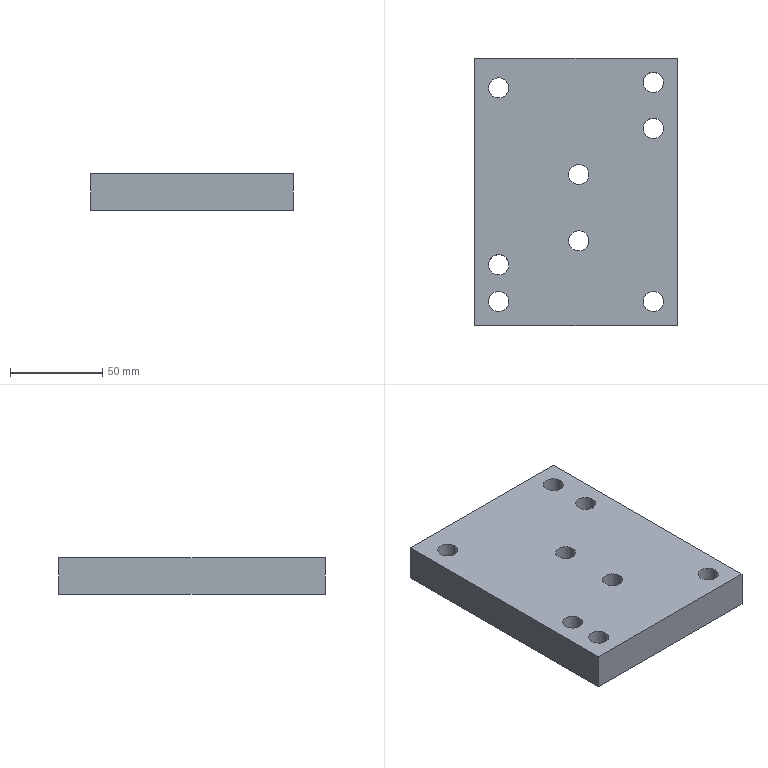Part | STEP file | 109_id3170_x_t | 1 solid | 14 faces | box 110 x 145 x 20 mm | volume 303795 mm3 | cylinder 8 | plane 6 | commonest cylinder face diameters 11 x8
STEP:
#1=CARTESIAN_POINT('',(0.,0.,0.));
#2=DIRECTION('',(0.,0.,1.));
#3=DIRECTION('',(1.,0.,0.));
#4=AXIS2_PLACEMENT_3D('',#1,#2,#3);
#5=CARTESIAN_POINT('',(-312.,-123.,105.));
#6=VERTEX_POINT('',#5);
#7=CARTESIAN_POINT('',(-317.5,-123.,105.));
#8=DIRECTION('',(0.,0.,1.));
#9=DIRECTION('',(1.,0.,0.));
#10=AXIS2_PLACEMENT_3D('',#7,#8,#9);
#11=CIRCLE('',#10,5.5);
#12=CARTESIAN_POINT('',(-319.,-95.5,105.));
#13=DIRECTION('',(0.,0.,1.));
#14=DIRECTION('',(-1.,0.,0.));
#15=AXIS2_PLACEMENT_3D('',#12,#13,#14);
#16=PLANE('',#15);
#17=CARTESIAN_POINT('',(-1.5,27.5));
#18=DIRECTION('',(-1.,0.));
#19=AXIS2_PLACEMENT_2D('',#17,#18);
#20=CIRCLE('',#19,5.5);
#21=(GEOMETRIC_REPRESENTATION_CONTEXT(2)PARAMETRIC_REPRESENTATION_CONTEXT()REPRESENTATION_CONTEXT('',''));
#22=DEFINITIONAL_REPRESENTATION('',(#20),#21);
#23=PCURVE('',#16,#22);
#24=CARTESIAN_POINT('',(-317.5,-123.,289.));
#25=DIRECTION('',(0.,0.,-1.));
#26=DIRECTION('',(1.,0.,0.));
#27=AXIS2_PLACEMENT_3D('',#24,#25,#26);
#28=CYLINDRICAL_SURFACE('',#27,5.5);
#29=CARTESIAN_POINT('',(6.283,184.));
#30=DIRECTION('',(-1.,0.));
#31=VECTOR('',#30,1.);
#32=LINE('',#29,#31);
#33=(GEOMETRIC_REPRESENTATION_CONTEXT(2)PARAMETRIC_REPRESENTATION_CONTEXT()REPRESENTATION_CONTEXT('',''));
#34=DEFINITIONAL_REPRESENTATION('',(#32),#33);
#35=PCURVE('',#28,#34);
#36=SURFACE_CURVE('',#11,(#23,#35),.PCURVE_S1.);
#37=EDGE_CURVE('',#6,#6,#36,.T.);
#38=ORIENTED_EDGE('',*,*,#37,.F.);
#39=EDGE_LOOP('',(#38));
#40=FACE_BOUND('',#39,.T.);
#41=CARTESIAN_POINT('',(-312.,-87.,105.));
#42=VERTEX_POINT('',#41);
#43=CARTESIAN_POINT('',(-317.5,-87.,105.));
#44=DIRECTION('',(0.,0.,1.));
#45=DIRECTION('',(1.,0.,0.));
#46=AXIS2_PLACEMENT_3D('',#43,#44,#45);
#47=CIRCLE('',#46,5.5);
#48=CARTESIAN_POINT('',(-1.5,-8.5));
#49=DIRECTION('',(-1.,0.));
#50=AXIS2_PLACEMENT_2D('',#48,#49);
#51=CIRCLE('',#50,5.5);
#52=(GEOMETRIC_REPRESENTATION_CONTEXT(2)PARAMETRIC_REPRESENTATION_CONTEXT()REPRESENTATION_CONTEXT('',''));
#53=DEFINITIONAL_REPRESENTATION('',(#51),#52);
#54=PCURVE('',#16,#53);
#55=CARTESIAN_POINT('',(-317.5,-87.,289.));
#56=DIRECTION('',(0.,0.,-1.));
#57=DIRECTION('',(1.,0.,0.));
#58=AXIS2_PLACEMENT_3D('',#55,#56,#57);
#59=CYLINDRICAL_SURFACE('',#58,5.5);
#60=CARTESIAN_POINT('',(6.283,184.));
#61=DIRECTION('',(-1.,0.));
#62=VECTOR('',#61,1.);
#63=LINE('',#60,#62);
#64=(GEOMETRIC_REPRESENTATION_CONTEXT(2)PARAMETRIC_REPRESENTATION_CONTEXT()REPRESENTATION_CONTEXT('',''));
#65=DEFINITIONAL_REPRESENTATION('',(#63),#64);
#66=PCURVE('',#59,#65);
#67=SURFACE_CURVE('',#47,(#54,#66),.PCURVE_S1.);
#68=EDGE_CURVE('',#42,#42,#67,.T.);
#69=ORIENTED_EDGE('',*,*,#68,.F.);
#70=EDGE_LOOP('',(#69));
#71=FACE_BOUND('',#70,.T.);
#72=CARTESIAN_POINT('',(-355.5,-136.,105.));
#73=VERTEX_POINT('',#72);
#74=CARTESIAN_POINT('',(-361.,-136.,105.));
#75=DIRECTION('',(0.,0.,-1.));
#76=DIRECTION('',(1.,0.,0.));
#77=AXIS2_PLACEMENT_3D('',#74,#75,#76);
#78=CIRCLE('',#77,5.5);
#79=CARTESIAN_POINT('',(36.5,40.5));
#80=CARTESIAN_POINT('',(36.5,50.026));
#81=CARTESIAN_POINT('',(44.75,45.263));
#82=CARTESIAN_POINT('',(53.,40.5));
#83=CARTESIAN_POINT('',(44.75,35.737));
#84=CARTESIAN_POINT('',(36.5,30.974));
#85=CARTESIAN_POINT('',(36.5,40.5));
#86=(BOUNDED_CURVE()B_SPLINE_CURVE(2,(#79,#80,#81,#82,#83,#84,#85),.UNSPECIFIED.,.T.,.F.)B_SPLINE_CURVE_WITH_KNOTS((1,2,2,2,2,1),(-2.094,0.,2.094,4.189,6.283,8.378),.UNSPECIFIED.)CURVE()GEOMETRIC_REPRESENTATION_ITEM()RATIONAL_B_SPLINE_CURVE((1.,0.5,1.,0.5,1.,0.5,1.))REPRESENTATION_ITEM(''));
#87=(GEOMETRIC_REPRESENTATION_CONTEXT(2)PARAMETRIC_REPRESENTATION_CONTEXT()REPRESENTATION_CONTEXT('',''));
#88=DEFINITIONAL_REPRESENTATION('',(#86),#87);
#89=PCURVE('',#16,#88);
#90=CARTESIAN_POINT('',(-361.,-136.,90.));
#91=DIRECTION('',(0.,0.,1.));
#92=DIRECTION('',(-1.,0.,0.));
#93=AXIS2_PLACEMENT_3D('',#90,#91,#92);
#94=CYLINDRICAL_SURFACE('',#93,5.5);
#95=CARTESIAN_POINT('',(9.425,15.));
#96=DIRECTION('',(-1.,0.));
#97=VECTOR('',#96,1.);
#98=LINE('',#95,#97);
#99=(GEOMETRIC_REPRESENTATION_CONTEXT(2)PARAMETRIC_REPRESENTATION_CONTEXT()REPRESENTATION_CONTEXT('',''));
#100=DEFINITIONAL_REPRESENTATION('',(#98),#99);
#101=PCURVE('',#94,#100);
#102=SURFACE_CURVE('',#78,(#89,#101),.PCURVE_S1.);
#103=EDGE_CURVE('',#73,#73,#102,.T.);
#104=ORIENTED_EDGE('',*,*,#103,.T.);
#105=EDGE_LOOP('',(#104));
#106=FACE_BOUND('',#105,.T.);
#107=CARTESIAN_POINT('',(-271.5,-37.,105.));
#108=VERTEX_POINT('',#107);
#109=CARTESIAN_POINT('',(-277.,-37.,105.));
#110=DIRECTION('',(0.,0.,-1.));
#111=DIRECTION('',(1.,0.,0.));
#112=AXIS2_PLACEMENT_3D('',#109,#110,#111);
#113=CIRCLE('',#112,5.5);
#114=CARTESIAN_POINT('',(-47.5,-58.5));
#115=CARTESIAN_POINT('',(-47.5,-48.974));
#116=CARTESIAN_POINT('',(-39.25,-53.737));
#117=CARTESIAN_POINT('',(-31.,-58.5));
#118=CARTESIAN_POINT('',(-39.25,-63.263));
#119=CARTESIAN_POINT('',(-47.5,-68.026));
#120=CARTESIAN_POINT('',(-47.5,-58.5));
#121=(BOUNDED_CURVE()B_SPLINE_CURVE(2,(#114,#115,#116,#117,#118,#119,#120),.UNSPECIFIED.,.T.,.F.)B_SPLINE_CURVE_WITH_KNOTS((1,2,2,2,2,1),(-2.094,0.,2.094,4.189,6.283,8.378),.UNSPECIFIED.)CURVE()GEOMETRIC_REPRESENTATION_ITEM()RATIONAL_B_SPLINE_CURVE((1.,0.5,1.,0.5,1.,0.5,1.))REPRESENTATION_ITEM(''));
#122=(GEOMETRIC_REPRESENTATION_CONTEXT(2)PARAMETRIC_REPRESENTATION_CONTEXT()REPRESENTATION_CONTEXT('',''));
#123=DEFINITIONAL_REPRESENTATION('',(#121),#122);
#124=PCURVE('',#16,#123);
#125=CARTESIAN_POINT('',(-277.,-37.,90.));
#126=DIRECTION('',(0.,0.,1.));
#127=DIRECTION('',(-1.,0.,0.));
#128=AXIS2_PLACEMENT_3D('',#125,#126,#127);
#129=CYLINDRICAL_SURFACE('',#128,5.5);
#130=CARTESIAN_POINT('',(9.425,15.));
#131=DIRECTION('',(-1.,0.));
#132=VECTOR('',#131,1.);
#133=LINE('',#130,#132);
#134=(GEOMETRIC_REPRESENTATION_CONTEXT(2)PARAMETRIC_REPRESENTATION_CONTEXT()REPRESENTATION_CONTEXT('',''));
#135=DEFINITIONAL_REPRESENTATION('',(#133),#134);
#136=PCURVE('',#129,#135);
#137=SURFACE_CURVE('',#113,(#124,#136),.PCURVE_S1.);
#138=EDGE_CURVE('',#108,#108,#137,.T.);
#139=ORIENTED_EDGE('',*,*,#138,.T.);
#140=EDGE_LOOP('',(#139));
#141=FACE_BOUND('',#140,.T.);
#142=CARTESIAN_POINT('',(-355.5,-156.,105.));
#143=VERTEX_POINT('',#142);
#144=CARTESIAN_POINT('',(-361.,-156.,105.));
#145=DIRECTION('',(0.,0.,-1.));
#146=DIRECTION('',(1.,0.,0.));
#147=AXIS2_PLACEMENT_3D('',#144,#145,#146);
#148=CIRCLE('',#147,5.5);
#149=CARTESIAN_POINT('',(36.5,60.5));
#150=CARTESIAN_POINT('',(36.5,70.026));
#151=CARTESIAN_POINT('',(44.75,65.263));
#152=CARTESIAN_POINT('',(53.,60.5));
#153=CARTESIAN_POINT('',(44.75,55.737));
#154=CARTESIAN_POINT('',(36.5,50.974));
#155=CARTESIAN_POINT('',(36.5,60.5));
#156=(BOUNDED_CURVE()B_SPLINE_CURVE(2,(#149,#150,#151,#152,#153,#154,#155),.UNSPECIFIED.,.T.,.F.)B_SPLINE_CURVE_WITH_KNOTS((1,2,2,2,2,1),(-2.094,0.,2.094,4.189,6.283,8.378),.UNSPECIFIED.)CURVE()GEOMETRIC_REPRESENTATION_ITEM()RATIONAL_B_SPLINE_CURVE((1.,0.5,1.,0.5,1.,0.5,1.))REPRESENTATION_ITEM(''));
#157=(GEOMETRIC_REPRESENTATION_CONTEXT(2)PARAMETRIC_REPRESENTATION_CONTEXT()REPRESENTATION_CONTEXT('',''));
#158=DEFINITIONAL_REPRESENTATION('',(#156),#157);
#159=PCURVE('',#16,#158);
#160=CARTESIAN_POINT('',(-361.,-156.,90.));
#161=DIRECTION('',(0.,0.,1.));
#162=DIRECTION('',(-1.,0.,0.));
#163=AXIS2_PLACEMENT_3D('',#160,#161,#162);
#164=CYLINDRICAL_SURFACE('',#163,5.5);
#165=CARTESIAN_POINT('',(9.425,15.));
#166=DIRECTION('',(-1.,0.));
#167=VECTOR('',#166,1.);
#168=LINE('',#165,#167);
#169=(GEOMETRIC_REPRESENTATION_CONTEXT(2)PARAMETRIC_REPRESENTATION_CONTEXT()REPRESENTATION_CONTEXT('',''));
#170=DEFINITIONAL_REPRESENTATION('',(#168),#169);
#171=PCURVE('',#164,#170);
#172=SURFACE_CURVE('',#148,(#159,#171),.PCURVE_S1.);
#173=EDGE_CURVE('',#143,#143,#172,.T.);
#174=ORIENTED_EDGE('',*,*,#173,.T.);
#175=EDGE_LOOP('',(#174));
#176=FACE_BOUND('',#175,.T.);
#177=CARTESIAN_POINT('',(-264.,-169.,105.));
#178=VERTEX_POINT('',#177);
#179=CARTESIAN_POINT('',(-374.,-169.,105.));
#180=VERTEX_POINT('',#179);
#181=CARTESIAN_POINT('',(-319.,-169.,105.));
#182=DIRECTION('',(-1.,0.,0.));
#183=VECTOR('',#182,1.);
#184=LINE('',#181,#183);
#185=CARTESIAN_POINT('',(0.,73.5));
#186=DIRECTION('',(1.,0.));
#187=VECTOR('',#186,1.);
#188=LINE('',#185,#187);
#189=(GEOMETRIC_REPRESENTATION_CONTEXT(2)PARAMETRIC_REPRESENTATION_CONTEXT()REPRESENTATION_CONTEXT('',''));
#190=DEFINITIONAL_REPRESENTATION('',(#188),#189);
#191=PCURVE('',#16,#190);
#192=CARTESIAN_POINT('',(-319.,-169.,90.));
#193=DIRECTION('',(0.,-1.,0.));
#194=DIRECTION('',(0.,0.,1.));
#195=AXIS2_PLACEMENT_3D('',#192,#193,#194);
#196=PLANE('',#195);
#197=CARTESIAN_POINT('',(15.,0.));
#198=DIRECTION('',(0.,1.));
#199=VECTOR('',#198,1.);
#200=LINE('',#197,#199);
#201=(GEOMETRIC_REPRESENTATION_CONTEXT(2)PARAMETRIC_REPRESENTATION_CONTEXT()REPRESENTATION_CONTEXT('',''));
#202=DEFINITIONAL_REPRESENTATION('',(#200),#201);
#203=PCURVE('',#196,#202);
#204=SURFACE_CURVE('',#184,(#191,#203),.PCURVE_S1.);
#205=EDGE_CURVE('',#178,#180,#204,.T.);
#206=ORIENTED_EDGE('',*,*,#205,.F.);
#207=CARTESIAN_POINT('',(-264.,-24.,105.));
#208=VERTEX_POINT('',#207);
#209=CARTESIAN_POINT('',(-264.,-95.5,105.));
#210=DIRECTION('',(0.,-1.,0.));
#211=VECTOR('',#210,1.);
#212=LINE('',#209,#211);
#213=CARTESIAN_POINT('',(-55.,0.));
#214=DIRECTION('',(0.,1.));
#215=VECTOR('',#214,1.);
#216=LINE('',#213,#215);
#217=(GEOMETRIC_REPRESENTATION_CONTEXT(2)PARAMETRIC_REPRESENTATION_CONTEXT()REPRESENTATION_CONTEXT('',''));
#218=DEFINITIONAL_REPRESENTATION('',(#216),#217);
#219=PCURVE('',#16,#218);
#220=CARTESIAN_POINT('',(-264.,-95.5,90.));
#221=DIRECTION('',(1.,0.,0.));
#222=DIRECTION('',(0.,0.,1.));
#223=AXIS2_PLACEMENT_3D('',#220,#221,#222);
#224=PLANE('',#223);
#225=CARTESIAN_POINT('',(15.,0.));
#226=DIRECTION('',(0.,1.));
#227=VECTOR('',#226,1.);
#228=LINE('',#225,#227);
#229=(GEOMETRIC_REPRESENTATION_CONTEXT(2)PARAMETRIC_REPRESENTATION_CONTEXT()REPRESENTATION_CONTEXT('',''));
#230=DEFINITIONAL_REPRESENTATION('',(#228),#229);
#231=PCURVE('',#224,#230);
#232=SURFACE_CURVE('',#212,(#219,#231),.PCURVE_S1.);
#233=EDGE_CURVE('',#208,#178,#232,.T.);
#234=ORIENTED_EDGE('',*,*,#233,.F.);
#235=CARTESIAN_POINT('',(-374.,-24.,105.));
#236=VERTEX_POINT('',#235);
#237=CARTESIAN_POINT('',(-319.,-24.,105.));
#238=DIRECTION('',(1.,0.,0.));
#239=VECTOR('',#238,1.);
#240=LINE('',#237,#239);
#241=CARTESIAN_POINT('',(0.,-71.5));
#242=DIRECTION('',(-1.,0.));
#243=VECTOR('',#242,1.);
#244=LINE('',#241,#243);
#245=(GEOMETRIC_REPRESENTATION_CONTEXT(2)PARAMETRIC_REPRESENTATION_CONTEXT()REPRESENTATION_CONTEXT('',''));
#246=DEFINITIONAL_REPRESENTATION('',(#244),#245);
#247=PCURVE('',#16,#246);
#248=CARTESIAN_POINT('',(-319.,-24.,90.));
#249=DIRECTION('',(0.,1.,0.));
#250=DIRECTION('',(0.,0.,-1.));
#251=AXIS2_PLACEMENT_3D('',#248,#249,#250);
#252=PLANE('',#251);
#253=CARTESIAN_POINT('',(-15.,0.));
#254=DIRECTION('',(0.,-1.));
#255=VECTOR('',#254,1.);
#256=LINE('',#253,#255);
#257=(GEOMETRIC_REPRESENTATION_CONTEXT(2)PARAMETRIC_REPRESENTATION_CONTEXT()REPRESENTATION_CONTEXT('',''));
#258=DEFINITIONAL_REPRESENTATION('',(#256),#257);
#259=PCURVE('',#252,#258);
#260=SURFACE_CURVE('',#240,(#247,#259),.PCURVE_S1.);
#261=EDGE_CURVE('',#236,#208,#260,.T.);
#262=ORIENTED_EDGE('',*,*,#261,.F.);
#263=CARTESIAN_POINT('',(-374.,-95.5,105.));
#264=DIRECTION('',(0.,1.,0.));
#265=VECTOR('',#264,1.);
#266=LINE('',#263,#265);
#267=CARTESIAN_POINT('',(55.,0.));
#268=DIRECTION('',(0.,-1.));
#269=VECTOR('',#268,1.);
#270=LINE('',#267,#269);
#271=(GEOMETRIC_REPRESENTATION_CONTEXT(2)PARAMETRIC_REPRESENTATION_CONTEXT()REPRESENTATION_CONTEXT('',''));
#272=DEFINITIONAL_REPRESENTATION('',(#270),#271);
#273=PCURVE('',#16,#272);
#274=CARTESIAN_POINT('',(-374.,-95.5,90.));
#275=DIRECTION('',(-1.,0.,0.));
#276=DIRECTION('',(0.,0.,-1.));
#277=AXIS2_PLACEMENT_3D('',#274,#275,#276);
#278=PLANE('',#277);
#279=CARTESIAN_POINT('',(-15.,0.));
#280=DIRECTION('',(0.,-1.));
#281=VECTOR('',#280,1.);
#282=LINE('',#279,#281);
#283=(GEOMETRIC_REPRESENTATION_CONTEXT(2)PARAMETRIC_REPRESENTATION_CONTEXT()REPRESENTATION_CONTEXT('',''));
#284=DEFINITIONAL_REPRESENTATION('',(#282),#283);
#285=PCURVE('',#278,#284);
#286=SURFACE_CURVE('',#266,(#273,#285),.PCURVE_S1.);
#287=EDGE_CURVE('',#180,#236,#286,.T.);
#288=ORIENTED_EDGE('',*,*,#287,.F.);
#289=EDGE_LOOP('',(#206,#234,#262,#288));
#290=FACE_BOUND('',#289,.T.);
#291=CARTESIAN_POINT('',(-271.5,-156.,105.));
#292=VERTEX_POINT('',#291);
#293=CARTESIAN_POINT('',(-277.,-156.,105.));
#294=DIRECTION('',(0.,0.,-1.));
#295=DIRECTION('',(1.,0.,0.));
#296=AXIS2_PLACEMENT_3D('',#293,#294,#295);
#297=CIRCLE('',#296,5.5);
#298=CARTESIAN_POINT('',(-47.5,60.5));
#299=CARTESIAN_POINT('',(-47.5,70.026));
#300=CARTESIAN_POINT('',(-39.25,65.263));
#301=CARTESIAN_POINT('',(-31.,60.5));
#302=CARTESIAN_POINT('',(-39.25,55.737));
#303=CARTESIAN_POINT('',(-47.5,50.974));
#304=CARTESIAN_POINT('',(-47.5,60.5));
#305=(BOUNDED_CURVE()B_SPLINE_CURVE(2,(#298,#299,#300,#301,#302,#303,#304),.UNSPECIFIED.,.T.,.F.)B_SPLINE_CURVE_WITH_KNOTS((1,2,2,2,2,1),(-2.094,0.,2.094,4.189,6.283,8.378),.UNSPECIFIED.)CURVE()GEOMETRIC_REPRESENTATION_ITEM()RATIONAL_B_SPLINE_CURVE((1.,0.5,1.,0.5,1.,0.5,1.))REPRESENTATION_ITEM(''));
#306=(GEOMETRIC_REPRESENTATION_CONTEXT(2)PARAMETRIC_REPRESENTATION_CONTEXT()REPRESENTATION_CONTEXT('',''));
#307=DEFINITIONAL_REPRESENTATION('',(#305),#306);
#308=PCURVE('',#16,#307);
#309=CARTESIAN_POINT('',(-277.,-156.,90.));
#310=DIRECTION('',(0.,0.,1.));
#311=DIRECTION('',(-1.,0.,0.));
#312=AXIS2_PLACEMENT_3D('',#309,#310,#311);
#313=CYLINDRICAL_SURFACE('',#312,5.5);
#314=CARTESIAN_POINT('',(9.425,15.));
#315=DIRECTION('',(-1.,0.));
#316=VECTOR('',#315,1.);
#317=LINE('',#314,#316);
#318=(GEOMETRIC_REPRESENTATION_CONTEXT(2)PARAMETRIC_REPRESENTATION_CONTEXT()REPRESENTATION_CONTEXT('',''));
#319=DEFINITIONAL_REPRESENTATION('',(#317),#318);
#320=PCURVE('',#313,#319);
#321=SURFACE_CURVE('',#297,(#308,#320),.PCURVE_S1.);
#322=EDGE_CURVE('',#292,#292,#321,.T.);
#323=ORIENTED_EDGE('',*,*,#322,.T.);
#324=EDGE_LOOP('',(#323));
#325=FACE_BOUND('',#324,.T.);
#326=CARTESIAN_POINT('',(-355.5,-40.,105.));
#327=VERTEX_POINT('',#326);
#328=CARTESIAN_POINT('',(-361.,-40.,105.));
#329=DIRECTION('',(0.,0.,-1.));
#330=DIRECTION('',(1.,0.,0.));
#331=AXIS2_PLACEMENT_3D('',#328,#329,#330);
#332=CIRCLE('',#331,5.5);
#333=CARTESIAN_POINT('',(36.5,-55.5));
#334=CARTESIAN_POINT('',(36.5,-45.974));
#335=CARTESIAN_POINT('',(44.75,-50.737));
#336=CARTESIAN_POINT('',(53.,-55.5));
#337=CARTESIAN_POINT('',(44.75,-60.263));
#338=CARTESIAN_POINT('',(36.5,-65.026));
#339=CARTESIAN_POINT('',(36.5,-55.5));
#340=(BOUNDED_CURVE()B_SPLINE_CURVE(2,(#333,#334,#335,#336,#337,#338,#339),.UNSPECIFIED.,.T.,.F.)B_SPLINE_CURVE_WITH_KNOTS((1,2,2,2,2,1),(-2.094,0.,2.094,4.189,6.283,8.378),.UNSPECIFIED.)CURVE()GEOMETRIC_REPRESENTATION_ITEM()RATIONAL_B_SPLINE_CURVE((1.,0.5,1.,0.5,1.,0.5,1.))REPRESENTATION_ITEM(''));
#341=(GEOMETRIC_REPRESENTATION_CONTEXT(2)PARAMETRIC_REPRESENTATION_CONTEXT()REPRESENTATION_CONTEXT('',''));
#342=DEFINITIONAL_REPRESENTATION('',(#340),#341);
#343=PCURVE('',#16,#342);
#344=CARTESIAN_POINT('',(-361.,-40.,90.));
#345=DIRECTION('',(0.,0.,1.));
#346=DIRECTION('',(-1.,0.,0.));
#347=AXIS2_PLACEMENT_3D('',#344,#345,#346);
#348=CYLINDRICAL_SURFACE('',#347,5.5);
#349=CARTESIAN_POINT('',(9.425,15.));
#350=DIRECTION('',(-1.,0.));
#351=VECTOR('',#350,1.);
#352=LINE('',#349,#351);
#353=(GEOMETRIC_REPRESENTATION_CONTEXT(2)PARAMETRIC_REPRESENTATION_CONTEXT()REPRESENTATION_CONTEXT('',''));
#354=DEFINITIONAL_REPRESENTATION('',(#352),#353);
#355=PCURVE('',#348,#354);
#356=SURFACE_CURVE('',#332,(#343,#355),.PCURVE_S1.);
#357=EDGE_CURVE('',#327,#327,#356,.T.);
#358=ORIENTED_EDGE('',*,*,#357,.T.);
#359=EDGE_LOOP('',(#358));
#360=FACE_BOUND('',#359,.T.);
#361=CARTESIAN_POINT('',(-271.5,-62.,105.));
#362=VERTEX_POINT('',#361);
#363=CARTESIAN_POINT('',(-277.,-62.,105.));
#364=DIRECTION('',(0.,0.,-1.));
#365=DIRECTION('',(1.,0.,0.));
#366=AXIS2_PLACEMENT_3D('',#363,#364,#365);
#367=CIRCLE('',#366,5.5);
#368=CARTESIAN_POINT('',(-47.5,-33.5));
#369=CARTESIAN_POINT('',(-47.5,-23.974));
#370=CARTESIAN_POINT('',(-39.25,-28.737));
#371=CARTESIAN_POINT('',(-31.,-33.5));
#372=CARTESIAN_POINT('',(-39.25,-38.263));
#373=CARTESIAN_POINT('',(-47.5,-43.026));
#374=CARTESIAN_POINT('',(-47.5,-33.5));
#375=(BOUNDED_CURVE()B_SPLINE_CURVE(2,(#368,#369,#370,#371,#372,#373,#374),.UNSPECIFIED.,.T.,.F.)B_SPLINE_CURVE_WITH_KNOTS((1,2,2,2,2,1),(-2.094,0.,2.094,4.189,6.283,8.378),.UNSPECIFIED.)CURVE()GEOMETRIC_REPRESENTATION_ITEM()RATIONAL_B_SPLINE_CURVE((1.,0.5,1.,0.5,1.,0.5,1.))REPRESENTATION_ITEM(''));
#376=(GEOMETRIC_REPRESENTATION_CONTEXT(2)PARAMETRIC_REPRESENTATION_CONTEXT()REPRESENTATION_CONTEXT('',''));
#377=DEFINITIONAL_REPRESENTATION('',(#375),#376);
#378=PCURVE('',#16,#377);
#379=CARTESIAN_POINT('',(-277.,-62.,90.));
#380=DIRECTION('',(0.,0.,1.));
#381=DIRECTION('',(-1.,0.,0.));
#382=AXIS2_PLACEMENT_3D('',#379,#380,#381);
#383=CYLINDRICAL_SURFACE('',#382,5.5);
#384=CARTESIAN_POINT('',(9.425,15.));
#385=DIRECTION('',(-1.,0.));
#386=VECTOR('',#385,1.);
#387=LINE('',#384,#386);
#388=(GEOMETRIC_REPRESENTATION_CONTEXT(2)PARAMETRIC_REPRESENTATION_CONTEXT()REPRESENTATION_CONTEXT('',''));
#389=DEFINITIONAL_REPRESENTATION('',(#387),#388);
#390=PCURVE('',#383,#389);
#391=SURFACE_CURVE('',#367,(#378,#390),.PCURVE_S1.);
#392=EDGE_CURVE('',#362,#362,#391,.T.);
#393=ORIENTED_EDGE('',*,*,#392,.T.);
#394=EDGE_LOOP('',(#393));
#395=FACE_BOUND('',#394,.T.);
#396=ADVANCED_FACE('',(#40,#71,#106,#141,#176,#290,#325,#360,#395),#16,.T.);
#397=CARTESIAN_POINT('',(-323.,-123.,85.));
#398=VERTEX_POINT('',#397);
#399=CARTESIAN_POINT('',(-312.,-123.,85.));
#400=VERTEX_POINT('',#399);
#401=CARTESIAN_POINT('',(-317.5,-123.,85.));
#402=DIRECTION('',(0.,0.,-1.));
#403=DIRECTION('',(-1.,0.,0.));
#404=AXIS2_PLACEMENT_3D('',#401,#402,#403);
#405=CIRCLE('',#404,5.5);
#406=CARTESIAN_POINT('',(-319.,-95.5,85.));
#407=DIRECTION('',(0.,0.,-1.));
#408=DIRECTION('',(1.,0.,0.));
#409=AXIS2_PLACEMENT_3D('',#406,#407,#408);
#410=PLANE('',#409);
#411=CARTESIAN_POINT('',(1.5,27.5));
#412=DIRECTION('',(-1.,0.));
#413=AXIS2_PLACEMENT_2D('',#411,#412);
#414=CIRCLE('',#413,5.5);
#415=(GEOMETRIC_REPRESENTATION_CONTEXT(2)PARAMETRIC_REPRESENTATION_CONTEXT()REPRESENTATION_CONTEXT('',''));
#416=DEFINITIONAL_REPRESENTATION('',(#414),#415);
#417=PCURVE('',#410,#416);
#418=CARTESIAN_POINT('',(3.142,204.));
#419=DIRECTION('',(1.,0.));
#420=VECTOR('',#419,1.);
#421=LINE('',#418,#420);
#422=(GEOMETRIC_REPRESENTATION_CONTEXT(2)PARAMETRIC_REPRESENTATION_CONTEXT()REPRESENTATION_CONTEXT('',''));
#423=DEFINITIONAL_REPRESENTATION('',(#421),#422);
#424=PCURVE('',#28,#423);
#425=SURFACE_CURVE('',#405,(#417,#424),.PCURVE_S1.);
#426=EDGE_CURVE('',#398,#400,#425,.T.);
#427=ORIENTED_EDGE('',*,*,#426,.F.);
#428=CARTESIAN_POINT('',(-317.5,-123.,85.));
#429=DIRECTION('',(0.,0.,-1.));
#430=DIRECTION('',(-1.,0.,0.));
#431=AXIS2_PLACEMENT_3D('',#428,#429,#430);
#432=CIRCLE('',#431,5.5);
#433=CARTESIAN_POINT('',(1.5,27.5));
#434=DIRECTION('',(-1.,0.));
#435=AXIS2_PLACEMENT_2D('',#433,#434);
#436=CIRCLE('',#435,5.5);
#437=(GEOMETRIC_REPRESENTATION_CONTEXT(2)PARAMETRIC_REPRESENTATION_CONTEXT()REPRESENTATION_CONTEXT('',''));
#438=DEFINITIONAL_REPRESENTATION('',(#436),#437);
#439=PCURVE('',#410,#438);
#440=CARTESIAN_POINT('',(-3.142,204.));
#441=DIRECTION('',(1.,0.));
#442=VECTOR('',#441,1.);
#443=LINE('',#440,#442);
#444=(GEOMETRIC_REPRESENTATION_CONTEXT(2)PARAMETRIC_REPRESENTATION_CONTEXT()REPRESENTATION_CONTEXT('',''));
#445=DEFINITIONAL_REPRESENTATION('',(#443),#444);
#446=PCURVE('',#28,#445);
#447=SURFACE_CURVE('',#432,(#439,#446),.PCURVE_S1.);
#448=EDGE_CURVE('',#400,#398,#447,.T.);
#449=ORIENTED_EDGE('',*,*,#448,.F.);
#450=EDGE_LOOP('',(#427,#449));
#451=FACE_BOUND('',#450,.T.);
#452=CARTESIAN_POINT('',(-323.,-87.,85.));
#453=VERTEX_POINT('',#452);
#454=CARTESIAN_POINT('',(-312.,-87.,85.));
#455=VERTEX_POINT('',#454);
#456=CARTESIAN_POINT('',(-317.5,-87.,85.));
#457=DIRECTION('',(0.,0.,-1.));
#458=DIRECTION('',(-1.,0.,0.));
#459=AXIS2_PLACEMENT_3D('',#456,#457,#458);
#460=CIRCLE('',#459,5.5);
#461=CARTESIAN_POINT('',(1.5,-8.5));
#462=DIRECTION('',(-1.,0.));
#463=AXIS2_PLACEMENT_2D('',#461,#462);
#464=CIRCLE('',#463,5.5);
#465=(GEOMETRIC_REPRESENTATION_CONTEXT(2)PARAMETRIC_REPRESENTATION_CONTEXT()REPRESENTATION_CONTEXT('',''));
#466=DEFINITIONAL_REPRESENTATION('',(#464),#465);
#467=PCURVE('',#410,#466);
#468=CARTESIAN_POINT('',(3.142,204.));
#469=DIRECTION('',(1.,0.));
#470=VECTOR('',#469,1.);
#471=LINE('',#468,#470);
#472=(GEOMETRIC_REPRESENTATION_CONTEXT(2)PARAMETRIC_REPRESENTATION_CONTEXT()REPRESENTATION_CONTEXT('',''));
#473=DEFINITIONAL_REPRESENTATION('',(#471),#472);
#474=PCURVE('',#59,#473);
#475=SURFACE_CURVE('',#460,(#467,#474),.PCURVE_S1.);
#476=EDGE_CURVE('',#453,#455,#475,.T.);
#477=ORIENTED_EDGE('',*,*,#476,.F.);
#478=CARTESIAN_POINT('',(-317.5,-87.,85.));
#479=DIRECTION('',(0.,0.,-1.));
#480=DIRECTION('',(-1.,0.,0.));
#481=AXIS2_PLACEMENT_3D('',#478,#479,#480);
#482=CIRCLE('',#481,5.5);
#483=CARTESIAN_POINT('',(1.5,-8.5));
#484=DIRECTION('',(-1.,0.));
#485=AXIS2_PLACEMENT_2D('',#483,#484);
#486=CIRCLE('',#485,5.5);
#487=(GEOMETRIC_REPRESENTATION_CONTEXT(2)PARAMETRIC_REPRESENTATION_CONTEXT()REPRESENTATION_CONTEXT('',''));
#488=DEFINITIONAL_REPRESENTATION('',(#486),#487);
#489=PCURVE('',#410,#488);
#490=CARTESIAN_POINT('',(-3.142,204.));
#491=DIRECTION('',(1.,0.));
#492=VECTOR('',#491,1.);
#493=LINE('',#490,#492);
#494=(GEOMETRIC_REPRESENTATION_CONTEXT(2)PARAMETRIC_REPRESENTATION_CONTEXT()REPRESENTATION_CONTEXT('',''));
#495=DEFINITIONAL_REPRESENTATION('',(#493),#494);
#496=PCURVE('',#59,#495);
#497=SURFACE_CURVE('',#482,(#489,#496),.PCURVE_S1.);
#498=EDGE_CURVE('',#455,#453,#497,.T.);
#499=ORIENTED_EDGE('',*,*,#498,.F.);
#500=EDGE_LOOP('',(#477,#499));
#501=FACE_BOUND('',#500,.T.);
#502=CARTESIAN_POINT('',(-355.5,-136.,85.));
#503=VERTEX_POINT('',#502);
#504=CARTESIAN_POINT('',(-361.,-136.,85.));
#505=DIRECTION('',(0.,0.,1.));
#506=DIRECTION('',(-1.,0.,0.));
#507=AXIS2_PLACEMENT_3D('',#504,#505,#506);
#508=CIRCLE('',#507,5.5);
#509=CARTESIAN_POINT('',(-47.5,40.5));
#510=CARTESIAN_POINT('',(-47.5,50.026));
#511=CARTESIAN_POINT('',(-39.25,45.263));
#512=CARTESIAN_POINT('',(-31.,40.5));
#513=CARTESIAN_POINT('',(-39.25,35.737));
#514=CARTESIAN_POINT('',(-47.5,30.974));
#515=CARTESIAN_POINT('',(-47.5,40.5));
#516=(BOUNDED_CURVE()B_SPLINE_CURVE(2,(#509,#510,#511,#512,#513,#514,#515),.UNSPECIFIED.,.T.,.F.)B_SPLINE_CURVE_WITH_KNOTS((1,2,2,2,2,1),(-2.094,0.,2.094,4.189,6.283,8.378),.UNSPECIFIED.)CURVE()GEOMETRIC_REPRESENTATION_ITEM()RATIONAL_B_SPLINE_CURVE((1.,0.5,1.,0.5,1.,0.5,1.))REPRESENTATION_ITEM(''));
#517=(GEOMETRIC_REPRESENTATION_CONTEXT(2)PARAMETRIC_REPRESENTATION_CONTEXT()REPRESENTATION_CONTEXT('',''));
#518=DEFINITIONAL_REPRESENTATION('',(#516),#517);
#519=PCURVE('',#410,#518);
#520=CARTESIAN_POINT('',(0.,-5.));
#521=DIRECTION('',(1.,0.));
#522=VECTOR('',#521,1.);
#523=LINE('',#520,#522);
#524=(GEOMETRIC_REPRESENTATION_CONTEXT(2)PARAMETRIC_REPRESENTATION_CONTEXT()REPRESENTATION_CONTEXT('',''));
#525=DEFINITIONAL_REPRESENTATION('',(#523),#524);
#526=PCURVE('',#94,#525);
#527=SURFACE_CURVE('',#508,(#519,#526),.PCURVE_S1.);
#528=EDGE_CURVE('',#503,#503,#527,.T.);
#529=ORIENTED_EDGE('',*,*,#528,.T.);
#530=EDGE_LOOP('',(#529));
#531=FACE_BOUND('',#530,.T.);
#532=CARTESIAN_POINT('',(-271.5,-37.,85.));
#533=VERTEX_POINT('',#532);
#534=CARTESIAN_POINT('',(-277.,-37.,85.));
#535=DIRECTION('',(0.,0.,1.));
#536=DIRECTION('',(-1.,0.,0.));
#537=AXIS2_PLACEMENT_3D('',#534,#535,#536);
#538=CIRCLE('',#537,5.5);
#539=CARTESIAN_POINT('',(36.5,-58.5));
#540=CARTESIAN_POINT('',(36.5,-48.974));
#541=CARTESIAN_POINT('',(44.75,-53.737));
#542=CARTESIAN_POINT('',(53.,-58.5));
#543=CARTESIAN_POINT('',(44.75,-63.263));
#544=CARTESIAN_POINT('',(36.5,-68.026));
#545=CARTESIAN_POINT('',(36.5,-58.5));
#546=(BOUNDED_CURVE()B_SPLINE_CURVE(2,(#539,#540,#541,#542,#543,#544,#545),.UNSPECIFIED.,.T.,.F.)B_SPLINE_CURVE_WITH_KNOTS((1,2,2,2,2,1),(-2.094,0.,2.094,4.189,6.283,8.378),.UNSPECIFIED.)CURVE()GEOMETRIC_REPRESENTATION_ITEM()RATIONAL_B_SPLINE_CURVE((1.,0.5,1.,0.5,1.,0.5,1.))REPRESENTATION_ITEM(''));
#547=(GEOMETRIC_REPRESENTATION_CONTEXT(2)PARAMETRIC_REPRESENTATION_CONTEXT()REPRESENTATION_CONTEXT('',''));
#548=DEFINITIONAL_REPRESENTATION('',(#546),#547);
#549=PCURVE('',#410,#548);
#550=CARTESIAN_POINT('',(0.,-5.));
#551=DIRECTION('',(1.,0.));
#552=VECTOR('',#551,1.);
#553=LINE('',#550,#552);
#554=(GEOMETRIC_REPRESENTATION_CONTEXT(2)PARAMETRIC_REPRESENTATION_CONTEXT()REPRESENTATION_CONTEXT('',''));
#555=DEFINITIONAL_REPRESENTATION('',(#553),#554);
#556=PCURVE('',#129,#555);
#557=SURFACE_CURVE('',#538,(#549,#556),.PCURVE_S1.);
#558=EDGE_CURVE('',#533,#533,#557,.T.);
#559=ORIENTED_EDGE('',*,*,#558,.T.);
#560=EDGE_LOOP('',(#559));
#561=FACE_BOUND('',#560,.T.);
#562=CARTESIAN_POINT('',(-355.5,-156.,85.));
#563=VERTEX_POINT('',#562);
#564=CARTESIAN_POINT('',(-361.,-156.,85.));
#565=DIRECTION('',(0.,0.,1.));
#566=DIRECTION('',(-1.,0.,0.));
#567=AXIS2_PLACEMENT_3D('',#564,#565,#566);
#568=CIRCLE('',#567,5.5);
#569=CARTESIAN_POINT('',(-47.5,60.5));
#570=CARTESIAN_POINT('',(-47.5,70.026));
#571=CARTESIAN_POINT('',(-39.25,65.263));
#572=CARTESIAN_POINT('',(-31.,60.5));
#573=CARTESIAN_POINT('',(-39.25,55.737));
#574=CARTESIAN_POINT('',(-47.5,50.974));
#575=CARTESIAN_POINT('',(-47.5,60.5));
#576=(BOUNDED_CURVE()B_SPLINE_CURVE(2,(#569,#570,#571,#572,#573,#574,#575),.UNSPECIFIED.,.T.,.F.)B_SPLINE_CURVE_WITH_KNOTS((1,2,2,2,2,1),(-2.094,0.,2.094,4.189,6.283,8.378),.UNSPECIFIED.)CURVE()GEOMETRIC_REPRESENTATION_ITEM()RATIONAL_B_SPLINE_CURVE((1.,0.5,1.,0.5,1.,0.5,1.))REPRESENTATION_ITEM(''));
#577=(GEOMETRIC_REPRESENTATION_CONTEXT(2)PARAMETRIC_REPRESENTATION_CONTEXT()REPRESENTATION_CONTEXT('',''));
#578=DEFINITIONAL_REPRESENTATION('',(#576),#577);
#579=PCURVE('',#410,#578);
#580=CARTESIAN_POINT('',(0.,-5.));
#581=DIRECTION('',(1.,0.));
#582=VECTOR('',#581,1.);
#583=LINE('',#580,#582);
#584=(GEOMETRIC_REPRESENTATION_CONTEXT(2)PARAMETRIC_REPRESENTATION_CONTEXT()REPRESENTATION_CONTEXT('',''));
#585=DEFINITIONAL_REPRESENTATION('',(#583),#584);
#586=PCURVE('',#164,#585);
#587=SURFACE_CURVE('',#568,(#579,#586),.PCURVE_S1.);
#588=EDGE_CURVE('',#563,#563,#587,.T.);
#589=ORIENTED_EDGE('',*,*,#588,.T.);
#590=EDGE_LOOP('',(#589));
#591=FACE_BOUND('',#590,.T.);
#592=CARTESIAN_POINT('',(-264.,-169.,85.));
#593=VERTEX_POINT('',#592);
#594=CARTESIAN_POINT('',(-264.,-24.,85.));
#595=VERTEX_POINT('',#594);
#596=CARTESIAN_POINT('',(-264.,-95.5,85.));
#597=DIRECTION('',(0.,1.,0.));
#598=VECTOR('',#597,1.);
#599=LINE('',#596,#598);
#600=CARTESIAN_POINT('',(55.,0.));
#601=DIRECTION('',(0.,-1.));
#602=VECTOR('',#601,1.);
#603=LINE('',#600,#602);
#604=(GEOMETRIC_REPRESENTATION_CONTEXT(2)PARAMETRIC_REPRESENTATION_CONTEXT()REPRESENTATION_CONTEXT('',''));
#605=DEFINITIONAL_REPRESENTATION('',(#603),#604);
#606=PCURVE('',#410,#605);
#607=CARTESIAN_POINT('',(-5.,0.));
#608=DIRECTION('',(0.,-1.));
#609=VECTOR('',#608,1.);
#610=LINE('',#607,#609);
#611=(GEOMETRIC_REPRESENTATION_CONTEXT(2)PARAMETRIC_REPRESENTATION_CONTEXT()REPRESENTATION_CONTEXT('',''));
#612=DEFINITIONAL_REPRESENTATION('',(#610),#611);
#613=PCURVE('',#224,#612);
#614=SURFACE_CURVE('',#599,(#606,#613),.PCURVE_S1.);
#615=EDGE_CURVE('',#593,#595,#614,.T.);
#616=ORIENTED_EDGE('',*,*,#615,.F.);
#617=CARTESIAN_POINT('',(-374.,-169.,85.));
#618=VERTEX_POINT('',#617);
#619=CARTESIAN_POINT('',(-319.,-169.,85.));
#620=DIRECTION('',(1.,0.,0.));
#621=VECTOR('',#620,1.);
#622=LINE('',#619,#621);
#623=CARTESIAN_POINT('',(0.,73.5));
#624=DIRECTION('',(1.,0.));
#625=VECTOR('',#624,1.);
#626=LINE('',#623,#625);
#627=(GEOMETRIC_REPRESENTATION_CONTEXT(2)PARAMETRIC_REPRESENTATION_CONTEXT()REPRESENTATION_CONTEXT('',''));
#628=DEFINITIONAL_REPRESENTATION('',(#626),#627);
#629=PCURVE('',#410,#628);
#630=CARTESIAN_POINT('',(-5.,0.));
#631=DIRECTION('',(0.,-1.));
#632=VECTOR('',#631,1.);
#633=LINE('',#630,#632);
#634=(GEOMETRIC_REPRESENTATION_CONTEXT(2)PARAMETRIC_REPRESENTATION_CONTEXT()REPRESENTATION_CONTEXT('',''));
#635=DEFINITIONAL_REPRESENTATION('',(#633),#634);
#636=PCURVE('',#196,#635);
#637=SURFACE_CURVE('',#622,(#629,#636),.PCURVE_S1.);
#638=EDGE_CURVE('',#618,#593,#637,.T.);
#639=ORIENTED_EDGE('',*,*,#638,.F.);
#640=CARTESIAN_POINT('',(-374.,-24.,85.));
#641=VERTEX_POINT('',#640);
#642=CARTESIAN_POINT('',(-374.,-95.5,85.));
#643=DIRECTION('',(0.,-1.,0.));
#644=VECTOR('',#643,1.);
#645=LINE('',#642,#644);
#646=CARTESIAN_POINT('',(-55.,0.));
#647=DIRECTION('',(0.,1.));
#648=VECTOR('',#647,1.);
#649=LINE('',#646,#648);
#650=(GEOMETRIC_REPRESENTATION_CONTEXT(2)PARAMETRIC_REPRESENTATION_CONTEXT()REPRESENTATION_CONTEXT('',''));
#651=DEFINITIONAL_REPRESENTATION('',(#649),#650);
#652=PCURVE('',#410,#651);
#653=CARTESIAN_POINT('',(5.,0.));
#654=DIRECTION('',(0.,1.));
#655=VECTOR('',#654,1.);
#656=LINE('',#653,#655);
#657=(GEOMETRIC_REPRESENTATION_CONTEXT(2)PARAMETRIC_REPRESENTATION_CONTEXT()REPRESENTATION_CONTEXT('',''));
#658=DEFINITIONAL_REPRESENTATION('',(#656),#657);
#659=PCURVE('',#278,#658);
#660=SURFACE_CURVE('',#645,(#652,#659),.PCURVE_S1.);
#661=EDGE_CURVE('',#641,#618,#660,.T.);
#662=ORIENTED_EDGE('',*,*,#661,.F.);
#663=CARTESIAN_POINT('',(-319.,-24.,85.));
#664=DIRECTION('',(-1.,0.,0.));
#665=VECTOR('',#664,1.);
#666=LINE('',#663,#665);
#667=CARTESIAN_POINT('',(0.,-71.5));
#668=DIRECTION('',(-1.,0.));
#669=VECTOR('',#668,1.);
#670=LINE('',#667,#669);
#671=(GEOMETRIC_REPRESENTATION_CONTEXT(2)PARAMETRIC_REPRESENTATION_CONTEXT()REPRESENTATION_CONTEXT('',''));
#672=DEFINITIONAL_REPRESENTATION('',(#670),#671);
#673=PCURVE('',#410,#672);
#674=CARTESIAN_POINT('',(5.,0.));
#675=DIRECTION('',(0.,1.));
#676=VECTOR('',#675,1.);
#677=LINE('',#674,#676);
#678=(GEOMETRIC_REPRESENTATION_CONTEXT(2)PARAMETRIC_REPRESENTATION_CONTEXT()REPRESENTATION_CONTEXT('',''));
#679=DEFINITIONAL_REPRESENTATION('',(#677),#678);
#680=PCURVE('',#252,#679);
#681=SURFACE_CURVE('',#666,(#673,#680),.PCURVE_S1.);
#682=EDGE_CURVE('',#595,#641,#681,.T.);
#683=ORIENTED_EDGE('',*,*,#682,.F.);
#684=EDGE_LOOP('',(#616,#639,#662,#683));
#685=FACE_BOUND('',#684,.T.);
#686=CARTESIAN_POINT('',(-271.5,-156.,85.));
#687=VERTEX_POINT('',#686);
#688=CARTESIAN_POINT('',(-277.,-156.,85.));
#689=DIRECTION('',(0.,0.,1.));
#690=DIRECTION('',(-1.,0.,0.));
#691=AXIS2_PLACEMENT_3D('',#688,#689,#690);
#692=CIRCLE('',#691,5.5);
#693=CARTESIAN_POINT('',(36.5,60.5));
#694=CARTESIAN_POINT('',(36.5,70.026));
#695=CARTESIAN_POINT('',(44.75,65.263));
#696=CARTESIAN_POINT('',(53.,60.5));
#697=CARTESIAN_POINT('',(44.75,55.737));
#698=CARTESIAN_POINT('',(36.5,50.974));
#699=CARTESIAN_POINT('',(36.5,60.5));
#700=(BOUNDED_CURVE()B_SPLINE_CURVE(2,(#693,#694,#695,#696,#697,#698,#699),.UNSPECIFIED.,.T.,.F.)B_SPLINE_CURVE_WITH_KNOTS((1,2,2,2,2,1),(-2.094,0.,2.094,4.189,6.283,8.378),.UNSPECIFIED.)CURVE()GEOMETRIC_REPRESENTATION_ITEM()RATIONAL_B_SPLINE_CURVE((1.,0.5,1.,0.5,1.,0.5,1.))REPRESENTATION_ITEM(''));
#701=(GEOMETRIC_REPRESENTATION_CONTEXT(2)PARAMETRIC_REPRESENTATION_CONTEXT()REPRESENTATION_CONTEXT('',''));
#702=DEFINITIONAL_REPRESENTATION('',(#700),#701);
#703=PCURVE('',#410,#702);
#704=CARTESIAN_POINT('',(0.,-5.));
#705=DIRECTION('',(1.,0.));
#706=VECTOR('',#705,1.);
#707=LINE('',#704,#706);
#708=(GEOMETRIC_REPRESENTATION_CONTEXT(2)PARAMETRIC_REPRESENTATION_CONTEXT()REPRESENTATION_CONTEXT('',''));
#709=DEFINITIONAL_REPRESENTATION('',(#707),#708);
#710=PCURVE('',#313,#709);
#711=SURFACE_CURVE('',#692,(#703,#710),.PCURVE_S1.);
#712=EDGE_CURVE('',#687,#687,#711,.T.);
#713=ORIENTED_EDGE('',*,*,#712,.T.);
#714=EDGE_LOOP('',(#713));
#715=FACE_BOUND('',#714,.T.);
#716=CARTESIAN_POINT('',(-355.5,-40.,85.));
#717=VERTEX_POINT('',#716);
#718=CARTESIAN_POINT('',(-361.,-40.,85.));
#719=DIRECTION('',(0.,0.,1.));
#720=DIRECTION('',(-1.,0.,0.));
#721=AXIS2_PLACEMENT_3D('',#718,#719,#720);
#722=CIRCLE('',#721,5.5);
#723=CARTESIAN_POINT('',(-47.5,-55.5));
#724=CARTESIAN_POINT('',(-47.5,-45.974));
#725=CARTESIAN_POINT('',(-39.25,-50.737));
#726=CARTESIAN_POINT('',(-31.,-55.5));
#727=CARTESIAN_POINT('',(-39.25,-60.263));
#728=CARTESIAN_POINT('',(-47.5,-65.026));
#729=CARTESIAN_POINT('',(-47.5,-55.5));
#730=(BOUNDED_CURVE()B_SPLINE_CURVE(2,(#723,#724,#725,#726,#727,#728,#729),.UNSPECIFIED.,.T.,.F.)B_SPLINE_CURVE_WITH_KNOTS((1,2,2,2,2,1),(-2.094,0.,2.094,4.189,6.283,8.378),.UNSPECIFIED.)CURVE()GEOMETRIC_REPRESENTATION_ITEM()RATIONAL_B_SPLINE_CURVE((1.,0.5,1.,0.5,1.,0.5,1.))REPRESENTATION_ITEM(''));
#731=(GEOMETRIC_REPRESENTATION_CONTEXT(2)PARAMETRIC_REPRESENTATION_CONTEXT()REPRESENTATION_CONTEXT('',''));
#732=DEFINITIONAL_REPRESENTATION('',(#730),#731);
#733=PCURVE('',#410,#732);
#734=CARTESIAN_POINT('',(0.,-5.));
#735=DIRECTION('',(1.,0.));
#736=VECTOR('',#735,1.);
#737=LINE('',#734,#736);
#738=(GEOMETRIC_REPRESENTATION_CONTEXT(2)PARAMETRIC_REPRESENTATION_CONTEXT()REPRESENTATION_CONTEXT('',''));
#739=DEFINITIONAL_REPRESENTATION('',(#737),#738);
#740=PCURVE('',#348,#739);
#741=SURFACE_CURVE('',#722,(#733,#740),.PCURVE_S1.);
#742=EDGE_CURVE('',#717,#717,#741,.T.);
#743=ORIENTED_EDGE('',*,*,#742,.T.);
#744=EDGE_LOOP('',(#743));
#745=FACE_BOUND('',#744,.T.);
#746=CARTESIAN_POINT('',(-271.5,-62.,85.));
#747=VERTEX_POINT('',#746);
#748=CARTESIAN_POINT('',(-277.,-62.,85.));
#749=DIRECTION('',(0.,0.,1.));
#750=DIRECTION('',(-1.,0.,0.));
#751=AXIS2_PLACEMENT_3D('',#748,#749,#750);
#752=CIRCLE('',#751,5.5);
#753=CARTESIAN_POINT('',(36.5,-33.5));
#754=CARTESIAN_POINT('',(36.5,-23.974));
#755=CARTESIAN_POINT('',(44.75,-28.737));
#756=CARTESIAN_POINT('',(53.,-33.5));
#757=CARTESIAN_POINT('',(44.75,-38.263));
#758=CARTESIAN_POINT('',(36.5,-43.026));
#759=CARTESIAN_POINT('',(36.5,-33.5));
#760=(BOUNDED_CURVE()B_SPLINE_CURVE(2,(#753,#754,#755,#756,#757,#758,#759),.UNSPECIFIED.,.T.,.F.)B_SPLINE_CURVE_WITH_KNOTS((1,2,2,2,2,1),(-2.094,0.,2.094,4.189,6.283,8.378),.UNSPECIFIED.)CURVE()GEOMETRIC_REPRESENTATION_ITEM()RATIONAL_B_SPLINE_CURVE((1.,0.5,1.,0.5,1.,0.5,1.))REPRESENTATION_ITEM(''));
#761=(GEOMETRIC_REPRESENTATION_CONTEXT(2)PARAMETRIC_REPRESENTATION_CONTEXT()REPRESENTATION_CONTEXT('',''));
#762=DEFINITIONAL_REPRESENTATION('',(#760),#761);
#763=PCURVE('',#410,#762);
#764=CARTESIAN_POINT('',(0.,-5.));
#765=DIRECTION('',(1.,0.));
#766=VECTOR('',#765,1.);
#767=LINE('',#764,#766);
#768=(GEOMETRIC_REPRESENTATION_CONTEXT(2)PARAMETRIC_REPRESENTATION_CONTEXT()REPRESENTATION_CONTEXT('',''));
#769=DEFINITIONAL_REPRESENTATION('',(#767),#768);
#770=PCURVE('',#383,#769);
#771=SURFACE_CURVE('',#752,(#763,#770),.PCURVE_S1.);
#772=EDGE_CURVE('',#747,#747,#771,.T.);
#773=ORIENTED_EDGE('',*,*,#772,.T.);
#774=EDGE_LOOP('',(#773));
#775=FACE_BOUND('',#774,.T.);
#776=ADVANCED_FACE('',(#451,#501,#531,#561,#591,#685,#715,#745,#775),#410,.T.);
#777=CARTESIAN_POINT('',(-264.,-169.,90.));
#778=DIRECTION('',(0.,0.,1.));
#779=VECTOR('',#778,1.);
#780=LINE('',#777,#779);
#781=CARTESIAN_POINT('',(0.,-55.));
#782=DIRECTION('',(1.,0.));
#783=VECTOR('',#782,1.);
#784=LINE('',#781,#783);
#785=(GEOMETRIC_REPRESENTATION_CONTEXT(2)PARAMETRIC_REPRESENTATION_CONTEXT()REPRESENTATION_CONTEXT('',''));
#786=DEFINITIONAL_REPRESENTATION('',(#784),#785);
#787=PCURVE('',#196,#786);
#788=CARTESIAN_POINT('',(0.,73.5));
#789=DIRECTION('',(1.,0.));
#790=VECTOR('',#789,1.);
#791=LINE('',#788,#790);
#792=(GEOMETRIC_REPRESENTATION_CONTEXT(2)PARAMETRIC_REPRESENTATION_CONTEXT()REPRESENTATION_CONTEXT('',''));
#793=DEFINITIONAL_REPRESENTATION('',(#791),#792);
#794=PCURVE('',#224,#793);
#795=SURFACE_CURVE('',#780,(#787,#794),.PCURVE_S1.);
#796=EDGE_CURVE('',#593,#178,#795,.T.);
#797=ORIENTED_EDGE('',*,*,#796,.T.);
#798=ORIENTED_EDGE('',*,*,#205,.T.);
#799=CARTESIAN_POINT('',(-374.,-169.,90.));
#800=DIRECTION('',(0.,0.,1.));
#801=VECTOR('',#800,1.);
#802=LINE('',#799,#801);
#803=CARTESIAN_POINT('',(0.,55.));
#804=DIRECTION('',(1.,0.));
#805=VECTOR('',#804,1.);
#806=LINE('',#803,#805);
#807=(GEOMETRIC_REPRESENTATION_CONTEXT(2)PARAMETRIC_REPRESENTATION_CONTEXT()REPRESENTATION_CONTEXT('',''));
#808=DEFINITIONAL_REPRESENTATION('',(#806),#807);
#809=PCURVE('',#196,#808);
#810=CARTESIAN_POINT('',(0.,73.5));
#811=DIRECTION('',(-1.,0.));
#812=VECTOR('',#811,1.);
#813=LINE('',#810,#812);
#814=(GEOMETRIC_REPRESENTATION_CONTEXT(2)PARAMETRIC_REPRESENTATION_CONTEXT()REPRESENTATION_CONTEXT('',''));
#815=DEFINITIONAL_REPRESENTATION('',(#813),#814);
#816=PCURVE('',#278,#815);
#817=SURFACE_CURVE('',#802,(#809,#816),.PCURVE_S1.);
#818=EDGE_CURVE('',#618,#180,#817,.T.);
#819=ORIENTED_EDGE('',*,*,#818,.F.);
#820=ORIENTED_EDGE('',*,*,#638,.T.);
#821=EDGE_LOOP('',(#797,#798,#819,#820));
#822=FACE_BOUND('',#821,.T.);
#823=ADVANCED_FACE('',(#822),#196,.T.);
#824=ORIENTED_EDGE('',*,*,#818,.T.);
#825=ORIENTED_EDGE('',*,*,#287,.T.);
#826=CARTESIAN_POINT('',(-374.,-24.,90.));
#827=DIRECTION('',(0.,0.,1.));
#828=VECTOR('',#827,1.);
#829=LINE('',#826,#828);
#830=CARTESIAN_POINT('',(0.,-71.5));
#831=DIRECTION('',(-1.,0.));
#832=VECTOR('',#831,1.);
#833=LINE('',#830,#832);
#834=(GEOMETRIC_REPRESENTATION_CONTEXT(2)PARAMETRIC_REPRESENTATION_CONTEXT()REPRESENTATION_CONTEXT('',''));
#835=DEFINITIONAL_REPRESENTATION('',(#833),#834);
#836=PCURVE('',#278,#835);
#837=CARTESIAN_POINT('',(0.,55.));
#838=DIRECTION('',(-1.,0.));
#839=VECTOR('',#838,1.);
#840=LINE('',#837,#839);
#841=(GEOMETRIC_REPRESENTATION_CONTEXT(2)PARAMETRIC_REPRESENTATION_CONTEXT()REPRESENTATION_CONTEXT('',''));
#842=DEFINITIONAL_REPRESENTATION('',(#840),#841);
#843=PCURVE('',#252,#842);
#844=SURFACE_CURVE('',#829,(#836,#843),.PCURVE_S1.);
#845=EDGE_CURVE('',#641,#236,#844,.T.);
#846=ORIENTED_EDGE('',*,*,#845,.F.);
#847=ORIENTED_EDGE('',*,*,#661,.T.);
#848=EDGE_LOOP('',(#824,#825,#846,#847));
#849=FACE_BOUND('',#848,.T.);
#850=ADVANCED_FACE('',(#849),#278,.T.);
#851=ORIENTED_EDGE('',*,*,#845,.T.);
#852=ORIENTED_EDGE('',*,*,#261,.T.);
#853=CARTESIAN_POINT('',(-264.,-24.,90.));
#854=DIRECTION('',(0.,0.,1.));
#855=VECTOR('',#854,1.);
#856=LINE('',#853,#855);
#857=CARTESIAN_POINT('',(0.,-55.));
#858=DIRECTION('',(-1.,0.));
#859=VECTOR('',#858,1.);
#860=LINE('',#857,#859);
#861=(GEOMETRIC_REPRESENTATION_CONTEXT(2)PARAMETRIC_REPRESENTATION_CONTEXT()REPRESENTATION_CONTEXT('',''));
#862=DEFINITIONAL_REPRESENTATION('',(#860),#861);
#863=PCURVE('',#252,#862);
#864=CARTESIAN_POINT('',(0.,-71.5));
#865=DIRECTION('',(1.,0.));
#866=VECTOR('',#865,1.);
#867=LINE('',#864,#866);
#868=(GEOMETRIC_REPRESENTATION_CONTEXT(2)PARAMETRIC_REPRESENTATION_CONTEXT()REPRESENTATION_CONTEXT('',''));
#869=DEFINITIONAL_REPRESENTATION('',(#867),#868);
#870=PCURVE('',#224,#869);
#871=SURFACE_CURVE('',#856,(#863,#870),.PCURVE_S1.);
#872=EDGE_CURVE('',#595,#208,#871,.T.);
#873=ORIENTED_EDGE('',*,*,#872,.F.);
#874=ORIENTED_EDGE('',*,*,#682,.T.);
#875=EDGE_LOOP('',(#851,#852,#873,#874));
#876=FACE_BOUND('',#875,.T.);
#877=ADVANCED_FACE('',(#876),#252,.T.);
#878=ORIENTED_EDGE('',*,*,#615,.T.);
#879=ORIENTED_EDGE('',*,*,#872,.T.);
#880=ORIENTED_EDGE('',*,*,#233,.T.);
#881=ORIENTED_EDGE('',*,*,#796,.F.);
#882=EDGE_LOOP('',(#878,#879,#880,#881));
#883=FACE_BOUND('',#882,.T.);
#884=ADVANCED_FACE('',(#883),#224,.T.);
#885=ORIENTED_EDGE('',*,*,#173,.T.);
#886=CARTESIAN_POINT('',(-355.5,-156.,85.));
#887=CARTESIAN_POINT('',(-355.5,-156.,105.));
#888=B_SPLINE_CURVE_WITH_KNOTS('',1,(#886,#887),.UNSPECIFIED.,.F.,.F.,(2,2),(-5.,15.),.PIECEWISE_BEZIER_KNOTS.);
#889=CARTESIAN_POINT('',(3.142,0.));
#890=DIRECTION('',(0.,1.));
#891=VECTOR('',#890,1.);
#892=LINE('',#889,#891);
#893=(GEOMETRIC_REPRESENTATION_CONTEXT(2)PARAMETRIC_REPRESENTATION_CONTEXT()REPRESENTATION_CONTEXT('',''));
#894=DEFINITIONAL_REPRESENTATION('',(#892),#893);
#895=PCURVE('',#164,#894);
#896=CARTESIAN_POINT('',(9.425,0.));
#897=DIRECTION('',(0.,1.));
#898=VECTOR('',#897,1.);
#899=LINE('',#896,#898);
#900=(GEOMETRIC_REPRESENTATION_CONTEXT(2)PARAMETRIC_REPRESENTATION_CONTEXT()REPRESENTATION_CONTEXT('',''));
#901=DEFINITIONAL_REPRESENTATION('',(#899),#900);
#902=PCURVE('',#164,#901);
#903=SEAM_CURVE('',#888,(#895,#902),.PCURVE_S1.);
#904=EDGE_CURVE('',#563,#143,#903,.T.);
#905=ORIENTED_EDGE('',*,*,#904,.F.);
#906=ORIENTED_EDGE('',*,*,#588,.T.);
#907=ORIENTED_EDGE('',*,*,#904,.T.);
#908=EDGE_LOOP('',(#885,#905,#906,#907));
#909=FACE_BOUND('',#908,.F.);
#910=ADVANCED_FACE('',(#909),#164,.F.);
#911=ORIENTED_EDGE('',*,*,#322,.T.);
#912=CARTESIAN_POINT('',(-271.5,-156.,85.));
#913=CARTESIAN_POINT('',(-271.5,-156.,105.));
#914=B_SPLINE_CURVE_WITH_KNOTS('',1,(#912,#913),.UNSPECIFIED.,.F.,.F.,(2,2),(-5.,15.),.PIECEWISE_BEZIER_KNOTS.);
#915=CARTESIAN_POINT('',(3.142,0.));
#916=DIRECTION('',(0.,1.));
#917=VECTOR('',#916,1.);
#918=LINE('',#915,#917);
#919=(GEOMETRIC_REPRESENTATION_CONTEXT(2)PARAMETRIC_REPRESENTATION_CONTEXT()REPRESENTATION_CONTEXT('',''));
#920=DEFINITIONAL_REPRESENTATION('',(#918),#919);
#921=PCURVE('',#313,#920);
#922=CARTESIAN_POINT('',(9.425,0.));
#923=DIRECTION('',(0.,1.));
#924=VECTOR('',#923,1.);
#925=LINE('',#922,#924);
#926=(GEOMETRIC_REPRESENTATION_CONTEXT(2)PARAMETRIC_REPRESENTATION_CONTEXT()REPRESENTATION_CONTEXT('',''));
#927=DEFINITIONAL_REPRESENTATION('',(#925),#926);
#928=PCURVE('',#313,#927);
#929=SEAM_CURVE('',#914,(#921,#928),.PCURVE_S1.);
#930=EDGE_CURVE('',#687,#292,#929,.T.);
#931=ORIENTED_EDGE('',*,*,#930,.F.);
#932=ORIENTED_EDGE('',*,*,#712,.T.);
#933=ORIENTED_EDGE('',*,*,#930,.T.);
#934=EDGE_LOOP('',(#911,#931,#932,#933));
#935=FACE_BOUND('',#934,.F.);
#936=ADVANCED_FACE('',(#935),#313,.F.);
#937=ORIENTED_EDGE('',*,*,#138,.T.);
#938=CARTESIAN_POINT('',(-271.5,-37.,85.));
#939=CARTESIAN_POINT('',(-271.5,-37.,105.));
#940=B_SPLINE_CURVE_WITH_KNOTS('',1,(#938,#939),.UNSPECIFIED.,.F.,.F.,(2,2),(-5.,15.),.PIECEWISE_BEZIER_KNOTS.);
#941=CARTESIAN_POINT('',(3.142,0.));
#942=DIRECTION('',(0.,1.));
#943=VECTOR('',#942,1.);
#944=LINE('',#941,#943);
#945=(GEOMETRIC_REPRESENTATION_CONTEXT(2)PARAMETRIC_REPRESENTATION_CONTEXT()REPRESENTATION_CONTEXT('',''));
#946=DEFINITIONAL_REPRESENTATION('',(#944),#945);
#947=PCURVE('',#129,#946);
#948=CARTESIAN_POINT('',(9.425,0.));
#949=DIRECTION('',(0.,1.));
#950=VECTOR('',#949,1.);
#951=LINE('',#948,#950);
#952=(GEOMETRIC_REPRESENTATION_CONTEXT(2)PARAMETRIC_REPRESENTATION_CONTEXT()REPRESENTATION_CONTEXT('',''));
#953=DEFINITIONAL_REPRESENTATION('',(#951),#952);
#954=PCURVE('',#129,#953);
#955=SEAM_CURVE('',#940,(#947,#954),.PCURVE_S1.);
#956=EDGE_CURVE('',#533,#108,#955,.T.);
#957=ORIENTED_EDGE('',*,*,#956,.F.);
#958=ORIENTED_EDGE('',*,*,#558,.T.);
#959=ORIENTED_EDGE('',*,*,#956,.T.);
#960=EDGE_LOOP('',(#937,#957,#958,#959));
#961=FACE_BOUND('',#960,.F.);
#962=ADVANCED_FACE('',(#961),#129,.F.);
#963=ORIENTED_EDGE('',*,*,#357,.T.);
#964=CARTESIAN_POINT('',(-355.5,-40.,85.));
#965=CARTESIAN_POINT('',(-355.5,-40.,105.));
#966=B_SPLINE_CURVE_WITH_KNOTS('',1,(#964,#965),.UNSPECIFIED.,.F.,.F.,(2,2),(-5.,15.),.PIECEWISE_BEZIER_KNOTS.);
#967=CARTESIAN_POINT('',(3.142,0.));
#968=DIRECTION('',(0.,1.));
#969=VECTOR('',#968,1.);
#970=LINE('',#967,#969);
#971=(GEOMETRIC_REPRESENTATION_CONTEXT(2)PARAMETRIC_REPRESENTATION_CONTEXT()REPRESENTATION_CONTEXT('',''));
#972=DEFINITIONAL_REPRESENTATION('',(#970),#971);
#973=PCURVE('',#348,#972);
#974=CARTESIAN_POINT('',(9.425,0.));
#975=DIRECTION('',(0.,1.));
#976=VECTOR('',#975,1.);
#977=LINE('',#974,#976);
#978=(GEOMETRIC_REPRESENTATION_CONTEXT(2)PARAMETRIC_REPRESENTATION_CONTEXT()REPRESENTATION_CONTEXT('',''));
#979=DEFINITIONAL_REPRESENTATION('',(#977),#978);
#980=PCURVE('',#348,#979);
#981=SEAM_CURVE('',#966,(#973,#980),.PCURVE_S1.);
#982=EDGE_CURVE('',#717,#327,#981,.T.);
#983=ORIENTED_EDGE('',*,*,#982,.F.);
#984=ORIENTED_EDGE('',*,*,#742,.T.);
#985=ORIENTED_EDGE('',*,*,#982,.T.);
#986=EDGE_LOOP('',(#963,#983,#984,#985));
#987=FACE_BOUND('',#986,.F.);
#988=ADVANCED_FACE('',(#987),#348,.F.);
#989=ORIENTED_EDGE('',*,*,#103,.T.);
#990=CARTESIAN_POINT('',(-355.5,-136.,85.));
#991=CARTESIAN_POINT('',(-355.5,-136.,105.));
#992=B_SPLINE_CURVE_WITH_KNOTS('',1,(#990,#991),.UNSPECIFIED.,.F.,.F.,(2,2),(-5.,15.),.PIECEWISE_BEZIER_KNOTS.);
#993=CARTESIAN_POINT('',(3.142,0.));
#994=DIRECTION('',(0.,1.));
#995=VECTOR('',#994,1.);
#996=LINE('',#993,#995);
#997=(GEOMETRIC_REPRESENTATION_CONTEXT(2)PARAMETRIC_REPRESENTATION_CONTEXT()REPRESENTATION_CONTEXT('',''));
#998=DEFINITIONAL_REPRESENTATION('',(#996),#997);
#999=PCURVE('',#94,#998);
#1000=CARTESIAN_POINT('',(9.425,0.));
#1001=DIRECTION('',(0.,1.));
#1002=VECTOR('',#1001,1.);
#1003=LINE('',#1000,#1002);
#1004=(GEOMETRIC_REPRESENTATION_CONTEXT(2)PARAMETRIC_REPRESENTATION_CONTEXT()REPRESENTATION_CONTEXT('',''));
#1005=DEFINITIONAL_REPRESENTATION('',(#1003),#1004);
#1006=PCURVE('',#94,#1005);
#1007=SEAM_CURVE('',#992,(#999,#1006),.PCURVE_S1.);
#1008=EDGE_CURVE('',#503,#73,#1007,.T.);
#1009=ORIENTED_EDGE('',*,*,#1008,.F.);
#1010=ORIENTED_EDGE('',*,*,#528,.T.);
#1011=ORIENTED_EDGE('',*,*,#1008,.T.);
#1012=EDGE_LOOP('',(#989,#1009,#1010,#1011));
#1013=FACE_BOUND('',#1012,.F.);
#1014=ADVANCED_FACE('',(#1013),#94,.F.);
#1015=ORIENTED_EDGE('',*,*,#392,.T.);
#1016=CARTESIAN_POINT('',(-271.5,-62.,85.));
#1017=CARTESIAN_POINT('',(-271.5,-62.,105.));
#1018=B_SPLINE_CURVE_WITH_KNOTS('',1,(#1016,#1017),.UNSPECIFIED.,.F.,.F.,(2,2),(-5.,15.),.PIECEWISE_BEZIER_KNOTS.);
#1019=CARTESIAN_POINT('',(3.142,0.));
#1020=DIRECTION('',(0.,1.));
#1021=VECTOR('',#1020,1.);
#1022=LINE('',#1019,#1021);
#1023=(GEOMETRIC_REPRESENTATION_CONTEXT(2)PARAMETRIC_REPRESENTATION_CONTEXT()REPRESENTATION_CONTEXT('',''));
#1024=DEFINITIONAL_REPRESENTATION('',(#1022),#1023);
#1025=PCURVE('',#383,#1024);
#1026=CARTESIAN_POINT('',(9.425,0.));
#1027=DIRECTION('',(0.,1.));
#1028=VECTOR('',#1027,1.);
#1029=LINE('',#1026,#1028);
#1030=(GEOMETRIC_REPRESENTATION_CONTEXT(2)PARAMETRIC_REPRESENTATION_CONTEXT()REPRESENTATION_CONTEXT('',''));
#1031=DEFINITIONAL_REPRESENTATION('',(#1029),#1030);
#1032=PCURVE('',#383,#1031);
#1033=SEAM_CURVE('',#1018,(#1025,#1032),.PCURVE_S1.);
#1034=EDGE_CURVE('',#747,#362,#1033,.T.);
#1035=ORIENTED_EDGE('',*,*,#1034,.F.);
#1036=ORIENTED_EDGE('',*,*,#772,.T.);
#1037=ORIENTED_EDGE('',*,*,#1034,.T.);
#1038=EDGE_LOOP('',(#1015,#1035,#1036,#1037));
#1039=FACE_BOUND('',#1038,.F.);
#1040=ADVANCED_FACE('',(#1039),#383,.F.);
#1041=ORIENTED_EDGE('',*,*,#68,.F.);
#1042=CARTESIAN_POINT('',(-312.,-87.,105.));
#1043=CARTESIAN_POINT('',(-312.,-87.,85.));
#1044=B_SPLINE_CURVE_WITH_KNOTS('',1,(#1042,#1043),.UNSPECIFIED.,.F.,.F.,(2,2),(184.,204.),.PIECEWISE_BEZIER_KNOTS.);
#1045=CARTESIAN_POINT('',(6.283,0.));
#1046=DIRECTION('',(0.,1.));
#1047=VECTOR('',#1046,1.);
#1048=LINE('',#1045,#1047);
#1049=(GEOMETRIC_REPRESENTATION_CONTEXT(2)PARAMETRIC_REPRESENTATION_CONTEXT()REPRESENTATION_CONTEXT('',''));
#1050=DEFINITIONAL_REPRESENTATION('',(#1048),#1049);
#1051=PCURVE('',#59,#1050);
#1052=CARTESIAN_POINT('',(0.,0.));
#1053=DIRECTION('',(0.,1.));
#1054=VECTOR('',#1053,1.);
#1055=LINE('',#1052,#1054);
#1056=(GEOMETRIC_REPRESENTATION_CONTEXT(2)PARAMETRIC_REPRESENTATION_CONTEXT()REPRESENTATION_CONTEXT('',''));
#1057=DEFINITIONAL_REPRESENTATION('',(#1055),#1056);
#1058=PCURVE('',#59,#1057);
#1059=SEAM_CURVE('',#1044,(#1051,#1058),.PCURVE_S1.);
#1060=EDGE_CURVE('',#42,#455,#1059,.T.);
#1061=ORIENTED_EDGE('',*,*,#1060,.T.);
#1062=ORIENTED_EDGE('',*,*,#476,.F.);
#1063=ORIENTED_EDGE('',*,*,#498,.F.);
#1064=ORIENTED_EDGE('',*,*,#1060,.F.);
#1065=EDGE_LOOP('',(#1041,#1061,#1062,#1063,#1064));
#1066=FACE_BOUND('',#1065,.F.);
#1067=ADVANCED_FACE('',(#1066),#59,.F.);
#1068=ORIENTED_EDGE('',*,*,#37,.F.);
#1069=CARTESIAN_POINT('',(-312.,-123.,105.));
#1070=CARTESIAN_POINT('',(-312.,-123.,85.));
#1071=B_SPLINE_CURVE_WITH_KNOTS('',1,(#1069,#1070),.UNSPECIFIED.,.F.,.F.,(2,2),(184.,204.),.PIECEWISE_BEZIER_KNOTS.);
#1072=CARTESIAN_POINT('',(6.283,0.));
#1073=DIRECTION('',(0.,1.));
#1074=VECTOR('',#1073,1.);
#1075=LINE('',#1072,#1074);
#1076=(GEOMETRIC_REPRESENTATION_CONTEXT(2)PARAMETRIC_REPRESENTATION_CONTEXT()REPRESENTATION_CONTEXT('',''));
#1077=DEFINITIONAL_REPRESENTATION('',(#1075),#1076);
#1078=PCURVE('',#28,#1077);
#1079=CARTESIAN_POINT('',(0.,0.));
#1080=DIRECTION('',(0.,1.));
#1081=VECTOR('',#1080,1.);
#1082=LINE('',#1079,#1081);
#1083=(GEOMETRIC_REPRESENTATION_CONTEXT(2)PARAMETRIC_REPRESENTATION_CONTEXT()REPRESENTATION_CONTEXT('',''));
#1084=DEFINITIONAL_REPRESENTATION('',(#1082),#1083);
#1085=PCURVE('',#28,#1084);
#1086=SEAM_CURVE('',#1071,(#1078,#1085),.PCURVE_S1.);
#1087=EDGE_CURVE('',#6,#400,#1086,.T.);
#1088=ORIENTED_EDGE('',*,*,#1087,.T.);
#1089=ORIENTED_EDGE('',*,*,#426,.F.);
#1090=ORIENTED_EDGE('',*,*,#448,.F.);
#1091=ORIENTED_EDGE('',*,*,#1087,.F.);
#1092=EDGE_LOOP('',(#1068,#1088,#1089,#1090,#1091));
#1093=FACE_BOUND('',#1092,.F.);
#1094=ADVANCED_FACE('',(#1093),#28,.F.);
#1095=CLOSED_SHELL('',(#396,#776,#823,#850,#877,#884,#910,#936,#962,#988,#1014,#1040,#1067,#1094));
#1096=MANIFOLD_SOLID_BREP('',#1095);
#1097=(LENGTH_UNIT()NAMED_UNIT(*)SI_UNIT(.MILLI.,.METRE.));
#1098=UNCERTAINTY_MEASURE_WITH_UNIT(LENGTH_MEASURE(0.000005),#1097,'','');
#1099=(NAMED_UNIT(*)PLANE_ANGLE_UNIT()SI_UNIT($,.RADIAN.));
#1100=(NAMED_UNIT(*)SI_UNIT($,.STERADIAN.)SOLID_ANGLE_UNIT());
#1101=(GEOMETRIC_REPRESENTATION_CONTEXT(3)GLOBAL_UNCERTAINTY_ASSIGNED_CONTEXT((#1098))GLOBAL_UNIT_ASSIGNED_CONTEXT((#1097,#1099,#1100))REPRESENTATION_CONTEXT('',''));
#1102=ADVANCED_BREP_SHAPE_REPRESENTATION('',(#4,#1096),#1101);